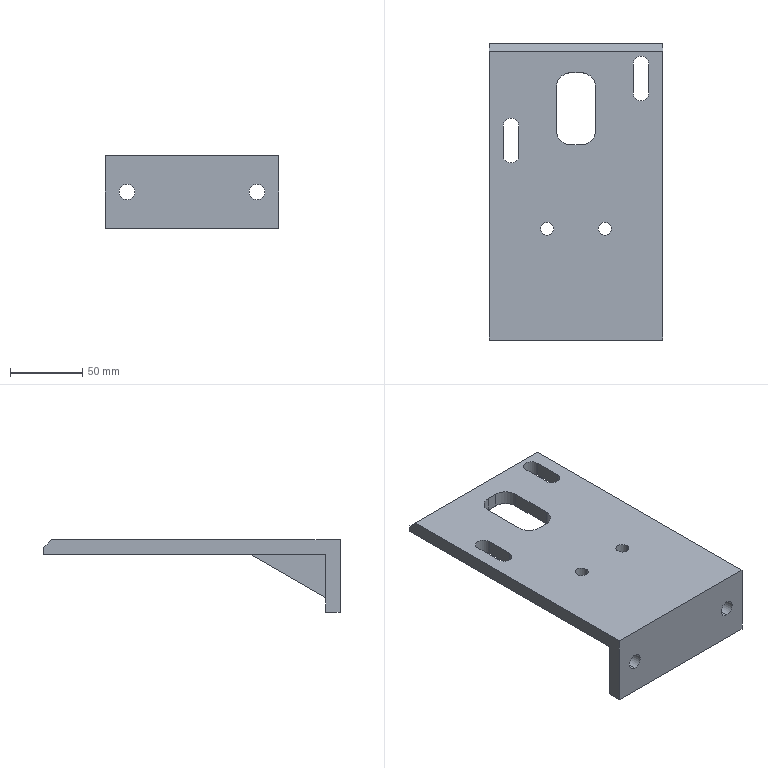NC program | NX | posted with a generic post | part box 120 x 205 x 50 mm
Lines 7209 to 8234 of 11006:
(ZLEVEL_PROFILE_COPY_1 , TOOL : D6)
N14404 T12 M6
N14406 G54
N14408 G17 G0 G90 X-88.106 Y29.874 B0. C0. S5000 M3
N14410 G43 Z30. H12
N14412 Z-10.85
N14414 G41 G94 G1 X-88.2 Y29.84 F1000. D12
N14416 X-89.1 Y29.321
N14418 G3 X-89.4 Y28.801 R0.6
N14420 G1 Y27.639
N14422 G3 X-88.8 Y27.621 R0.6
N14424 G1 X-87.999 Y28.052
N14426 G40
N14428 X-87.92 Y28.114
N14430 G0 X-88.106 Y30.399 Z-11.2
N14432 G41 G1 X-88.2 Y30.365
N14434 X-89.1 Y29.845
N14436 G3 X-89.4 Y29.326 R0.6
N14438 G1 Y27.936
N14440 G3 X-88.81 Y28.043 R0.6
N14442 G1 X-88.114 Y28.631
N14444 G40
N14446 X-88.05 Y28.708
N14448 G0 X-88.106 Y30.78 Z-11.55
N14450 G41 G1 X-88.2 Y30.746
N14452 X-89.1 Y30.226
N14454 G3 X-89.4 Y29.706 R0.6
N14456 G1 Y28.072
N14458 G3 X-88.845 Y28.299 R0.6
N14460 G1 X-88.2 Y29.133
N14462 G40
N14464 X-88.153 Y29.222
N14466 G0 X-88.106 Y31.059 Z-11.9
N14468 G41 G1 X-88.2 Y31.025
N14470 X-89.1 Y30.505
N14472 G3 X-89.4 Y29.986 R0.6
N14474 G1 Y28.099
N14476 X-89.283 Y28.1
N14478 X-89.209
N14480 G3 X-88.689 Y28.4 R0.6
N14482 G1 X-88.2 Y29.248
N14484 G40
N14486 X-88.166 Y29.342
N14488 G0 X-88.106 Y31.245 Z-12.25
N14490 G41 G1 X-88.2 Y31.211
N14492 X-89.1 Y30.692
N14494 G3 X-89.4 Y30.172 R0.6
N14496 G1 Y28.099
N14498 X-89.283 Y28.1
N14500 X-88.603
N14502 G3 X-88.083 Y28.4 R0.6
N14504 G1 X-87.628 Y29.188
N14506 G40
N14508 X-87.594 Y29.282
N14510 G0 X-88.106 Y31.354 Z-12.6
N14512 G41 G1 X-88.2 Y31.32
N14514 X-89.1 Y30.8
N14516 G3 X-89.4 Y30.28 R0.6
N14518 G1 Y28.099
N14520 X-89.283 Y28.1
N14522 X-87.997
N14524 G3 X-87.477 Y28.4 R0.6
N14526 G1 X-87.023 Y29.186
N14528 G40
N14530 X-86.989 Y29.28
N14532 G0 X-88.106 Y31.39 Z-12.95
N14534 G41 G1 X-88.2 Y31.356
N14536 X-89.1 Y30.836
N14538 G3 X-89.4 Y30.316 R0.6
N14540 G1 Y28.099
N14542 X-89.283 Y28.1
N14544 X-87.39
N14546 G3 X-86.871 Y28.4 R0.6
N14548 G1 X-86.417 Y29.186
N14550 G40
N14552 X-86.383 Y29.28
N14554 G0 X-88.106 Y31.39 Z-13.3
N14556 G41 G1 X-88.2 Y31.356
N14558 X-89.1 Y30.836
N14560 G3 X-89.4 Y30.316 R0.6
N14562 G1 Y28.099
N14564 X-89.283 Y28.1
N14566 X-87.184
N14568 G3 X-86.664 Y28.4 R0.6
N14570 G1 X-86.17 Y29.256
N14572 G40
N14574 X-86.136 Y29.35
N14576 G0 X-88.106 Y31.39 Z-13.65
N14578 G41 G1 X-88.2 Y31.356
N14580 X-89.1 Y30.836
N14582 G3 X-89.4 Y30.316 R0.6
N14584 G1 Y28.099
N14586 X-89.283 Y28.1
N14588 X-87.184
N14590 G3 X-86.664 Y28.4 R0.6
N14592 G1 X-86.144 Y29.3
N14594 G40
N14596 X-86.11 Y29.394
N14598 G0 X-88.106 Y31.39 Z-14.
N14600 G41 G1 X-88.2 Y31.356
N14602 X-89.1 Y30.836
N14604 G3 X-89.4 Y30.316 R0.6
N14606 G1 Y28.099
N14608 X-89.283 Y28.1
N14610 X-87.184
N14612 G3 X-86.664 Y28.4 R0.6
N14614 G1 X-86.144 Y29.3
N14616 G40
N14618 X-86.11 Y29.394
N14620 G0 X-88.106 Y31.39 Z-14.35
N14622 G41 G1 X-88.2 Y31.356
N14624 X-89.1 Y30.836
N14626 G3 X-89.4 Y30.316 R0.6
N14628 G1 Y28.099
N14630 X-89.283 Y28.1
N14632 X-87.184
N14634 G3 X-86.664 Y28.4 R0.6
N14636 G1 X-86.144 Y29.3
N14638 G40
N14640 X-86.11 Y29.394
N14642 G0 X-88.106 Y31.39 Z-14.7
N14644 G41 G1 X-88.2 Y31.356
N14646 X-89.1 Y30.836
N14648 G3 X-89.4 Y30.316 R0.6
N14650 G1 Y28.099
N14652 X-89.283 Y28.1
N14654 X-87.184
N14656 G3 X-86.664 Y28.4 R0.6
N14658 G1 X-86.144 Y29.3
N14660 G40
N14662 X-86.11 Y29.394
N14664 G0 X-88.106 Y31.39 Z-15.05
N14666 G41 G1 X-88.2 Y31.356
N14668 X-89.1 Y30.836
N14670 G3 X-89.4 Y30.316 R0.6
N14672 G1 Y28.099
N14674 X-89.283 Y28.1
N14676 X-87.184
N14678 G3 X-86.664 Y28.4 R0.6
N14680 G1 X-86.144 Y29.3
N14682 G40
N14684 X-86.11 Y29.394
N14686 G0 X-88.106 Y31.39 Z-15.4
N14688 G41 G1 X-88.2 Y31.356
N14690 X-89.1 Y30.836
N14692 G3 X-89.4 Y30.316 R0.6
N14694 G1 Y28.099
N14696 X-89.283 Y28.1
N14698 X-87.184
N14700 G3 X-86.664 Y28.4 R0.6
N14702 G1 X-86.144 Y29.3
N14704 G40
N14706 X-86.11 Y29.394
N14708 G0 X-88.106 Y31.39 Z-15.75
N14710 G41 G1 X-88.2 Y31.356
N14712 X-89.1 Y30.836
N14714 G3 X-89.4 Y30.316 R0.6
N14716 G1 Y28.099
N14718 X-89.283 Y28.1
N14720 X-87.184
N14722 G3 X-86.664 Y28.4 R0.6
N14724 G1 X-86.144 Y29.3
N14726 G40
N14728 X-86.11 Y29.394
N14730 G0 X-88.106 Y31.39 Z-16.1
N14732 G41 G1 X-88.2 Y31.356
N14734 X-89.1 Y30.836
N14736 G3 X-89.4 Y30.316 R0.6
N14738 G1 Y28.099
N14740 X-89.283 Y28.1
N14742 X-87.184
N14744 G3 X-86.664 Y28.4 R0.6
N14746 G1 X-86.144 Y29.3
N14748 G40
N14750 X-86.11 Y29.394
N14752 G0 X-88.106 Y31.39 Z-16.45
N14754 G41 G1 X-88.2 Y31.356
N14756 X-89.1 Y30.836
N14758 G3 X-89.4 Y30.316 R0.6
N14760 G1 Y28.099
N14762 X-89.283 Y28.1
N14764 X-87.184
N14766 G3 X-86.664 Y28.4 R0.6
N14768 G1 X-86.144 Y29.3
N14770 G40
N14772 X-86.11 Y29.394
N14774 G0 X-88.106 Y31.39 Z-16.8
N14776 G41 G1 X-88.2 Y31.356
N14778 X-89.1 Y30.836
N14780 G3 X-89.4 Y30.316 R0.6
N14782 G1 Y28.099
N14784 X-89.283 Y28.1
N14786 X-87.184
N14788 G3 X-86.664 Y28.4 R0.6
N14790 G1 X-86.144 Y29.3
N14792 G40
N14794 X-86.11 Y29.394
N14796 G0 X-88.106 Y31.39 Z-17.15
N14798 G41 G1 X-88.2 Y31.356
N14800 X-89.1 Y30.836
N14802 G3 X-89.4 Y30.316 R0.6
N14804 G1 Y28.099
N14806 X-89.283 Y28.1
N14808 X-87.184
N14810 G3 X-86.664 Y28.4 R0.6
N14812 G1 X-86.144 Y29.3
N14814 G40
N14816 X-86.11 Y29.394
N14818 G0 X-88.106 Y31.39 Z-17.5
N14820 G41 G1 X-88.2 Y31.356
N14822 X-89.1 Y30.836
N14824 G3 X-89.4 Y30.316 R0.6
N14826 G1 Y28.099
N14828 X-89.283 Y28.1
N14830 X-87.184
N14832 G3 X-86.664 Y28.4 R0.6
N14834 G1 X-86.144 Y29.3
N14836 G40
N14838 X-86.11 Y29.394
N14840 G0 X-88.106 Y31.39 Z-17.85
N14842 G41 G1 X-88.2 Y31.356
N14844 X-89.1 Y30.836
N14846 G3 X-89.4 Y30.316 R0.6
N14848 G1 Y28.099
N14850 X-89.283 Y28.1
N14852 X-87.184
N14854 G3 X-86.664 Y28.4 R0.6
N14856 G1 X-86.144 Y29.3
N14858 G40
N14860 X-86.11 Y29.394
N14862 G0 X-88.106 Y31.39 Z-18.2
N14864 G41 G1 X-88.2 Y31.356
N14866 X-89.1 Y30.836
N14868 G3 X-89.4 Y30.316 R0.6
N14870 G1 Y28.099
N14872 X-89.283 Y28.1
N14874 X-87.184
N14876 G3 X-86.664 Y28.4 R0.6
N14878 G1 X-86.144 Y29.3
N14880 G40
N14882 X-86.11 Y29.394
N14884 G0 X-88.106 Y31.39 Z-18.55
N14886 G41 G1 X-88.2 Y31.356
N14888 X-89.1 Y30.836
N14890 G3 X-89.4 Y30.316 R0.6
N14892 G1 Y28.099
N14894 X-89.283 Y28.1
N14896 X-87.184
N14898 G3 X-86.664 Y28.4 R0.6
N14900 G1 X-86.144 Y29.3
N14902 G40
N14904 X-86.11 Y29.394
N14906 G0 X-88.106 Y31.39 Z-18.9
N14908 G41 G1 X-88.2 Y31.356
N14910 X-89.1 Y30.836
N14912 G3 X-89.4 Y30.316 R0.6
N14914 G1 Y28.099
N14916 X-89.283 Y28.1
N14918 X-87.184
N14920 G3 X-86.664 Y28.4 R0.6
N14922 G1 X-86.144 Y29.3
N14924 G40
N14926 X-86.11 Y29.394
N14928 G0 X-88.106 Y31.39 Z-19.25
N14930 G41 G1 X-88.2 Y31.356
N14932 X-89.1 Y30.836
N14934 G3 X-89.4 Y30.316 R0.6
N14936 G1 Y28.099
N14938 X-89.283 Y28.1
N14940 X-87.184
N14942 G3 X-86.664 Y28.4 R0.6
N14944 G1 X-86.144 Y29.3
N14946 G40
N14948 X-86.11 Y29.394
N14950 G0 X-88.106 Y31.39 Z-19.6
N14952 G41 G1 X-88.2 Y31.356
N14954 X-89.1 Y30.836
N14956 G3 X-89.4 Y30.316 R0.6
N14958 G1 Y28.099
N14960 X-89.283 Y28.1
N14962 X-87.184
N14964 G3 X-86.664 Y28.4 R0.6
N14966 G1 X-86.144 Y29.3
N14968 G40
N14970 X-86.11 Y29.394
N14972 G0 X-88.106 Y31.39 Z-19.95
N14974 G41 G1 X-88.2 Y31.356
N14976 X-89.1 Y30.836
N14978 G3 X-89.4 Y30.316 R0.6
N14980 G1 Y28.099
N14982 X-89.283 Y28.1
N14984 X-87.184
N14986 G3 X-86.664 Y28.4 R0.6
N14988 G1 X-86.144 Y29.3
N14990 G40
N14992 X-86.11 Y29.394
N14994 G0 X-88.106 Y31.39 Z-20.3
N14996 G41 G1 X-88.2 Y31.356
N14998 X-89.1 Y30.836
N15000 G3 X-89.4 Y30.316 R0.6
N15002 G1 Y28.099
N15004 X-89.283 Y28.1
N15006 X-87.184
N15008 G3 X-86.664 Y28.4 R0.6
N15010 G1 X-86.144 Y29.3
N15012 G40
N15014 X-86.11 Y29.394
N15016 G0 X-88.106 Y31.39 Z-20.65
N15018 G41 G1 X-88.2 Y31.356
N15020 X-89.1 Y30.836
N15022 G3 X-89.4 Y30.316 R0.6
N15024 G1 Y28.099
N15026 X-89.283 Y28.1
N15028 X-87.184
N15030 G3 X-86.664 Y28.4 R0.6
N15032 G1 X-86.144 Y29.3
N15034 G40
N15036 X-86.11 Y29.394
N15038 G0 X-88.106 Y31.39 Z-21.
N15040 G41 G1 X-88.2 Y31.356
N15042 X-89.1 Y30.836
N15044 G3 X-89.4 Y30.316 R0.6
N15046 G1 Y28.099
N15048 X-89.283 Y28.1
N15050 X-87.184
N15052 G3 X-86.664 Y28.4 R0.6
N15054 G1 X-86.144 Y29.3
N15056 G40
N15058 X-86.11 Y29.394
N15060 G0 X-88.106 Y31.39 Z-21.35
N15062 G41 G1 X-88.2 Y31.356
N15064 X-89.1 Y30.836
N15066 G3 X-89.4 Y30.316 R0.6
N15068 G1 Y28.099
N15070 X-89.283 Y28.1
N15072 X-87.184
N15074 G3 X-86.664 Y28.4 R0.6
N15076 G1 X-86.144 Y29.3
N15078 G40
N15080 X-86.11 Y29.394
N15082 G0 X-88.106 Y31.39 Z-21.7
N15084 G41 G1 X-88.2 Y31.356
N15086 X-89.1 Y30.836
N15088 G3 X-89.4 Y30.316 R0.6
N15090 G1 Y28.099
N15092 X-89.283 Y28.1
N15094 X-87.184
N15096 G3 X-86.664 Y28.4 R0.6
N15098 G1 X-86.144 Y29.3
N15100 G40
N15102 X-86.11 Y29.394
N15104 G0 X-88.106 Y31.39 Z-22.05
N15106 G41 G1 X-88.2 Y31.356
N15108 X-89.1 Y30.836
N15110 G3 X-89.4 Y30.316 R0.6
N15112 G1 Y28.099
N15114 X-89.283 Y28.1
N15116 X-87.184
N15118 G3 X-86.664 Y28.4 R0.6
N15120 G1 X-86.144 Y29.3
N15122 G40
N15124 X-86.11 Y29.394
N15126 G0 X-88.106 Y31.39 Z-22.4
N15128 G41 G1 X-88.2 Y31.356
N15130 X-89.1 Y30.836
N15132 G3 X-89.4 Y30.316 R0.6
N15134 G1 Y28.099
N15136 X-89.283 Y28.1
N15138 X-87.184
N15140 G3 X-86.664 Y28.4 R0.6
N15142 G1 X-86.144 Y29.3
N15144 G40
N15146 X-86.11 Y29.394
N15148 G0 X-88.106 Y31.39 Z-22.75
N15150 G41 G1 X-88.2 Y31.356
N15152 X-89.1 Y30.836
N15154 G3 X-89.4 Y30.316 R0.6
N15156 G1 Y28.099
N15158 X-89.283 Y28.1
N15160 X-87.184
N15162 G3 X-86.664 Y28.4 R0.6
N15164 G1 X-86.144 Y29.3
N15166 G40
N15168 X-86.11 Y29.394
N15170 G0 X-88.106 Y31.39 Z-23.1
N15172 G41 G1 X-88.2 Y31.356
N15174 X-89.1 Y30.836
N15176 G3 X-89.4 Y30.316 R0.6
N15178 G1 Y28.099
N15180 X-89.283 Y28.1
N15182 X-87.184
N15184 G3 X-86.664 Y28.4 R0.6
N15186 G1 X-86.144 Y29.3
N15188 G40
N15190 X-86.11 Y29.394
N15192 G0 X-88.106 Y31.39 Z-23.45
N15194 G41 G1 X-88.2 Y31.356
N15196 X-89.1 Y30.836
N15198 G3 X-89.4 Y30.316 R0.6
N15200 G1 Y28.1
N15202 X-89.283
N15204 X-87.184
N15206 G3 X-86.664 Y28.4 R0.6
N15208 G1 X-86.144 Y29.3
N15210 G40
N15212 X-86.11 Y29.394
N15214 G0 X-88.106 Y31.39 Z-23.8
N15216 G41 G1 X-88.2 Y31.356
N15218 X-89.1 Y30.836
N15220 G3 X-89.4 Y30.316 R0.6
N15222 G1 Y28.1
N15224 X-89.283
N15226 X-87.184
N15228 G3 X-86.664 Y28.4 R0.6
N15230 G1 X-86.144 Y29.3
N15232 G40
N15234 X-86.11 Y29.394
N15236 G0 X-88.106 Y31.39 Z-24.15
N15238 G41 G1 X-88.2 Y31.356
N15240 X-89.1 Y30.836
N15242 G3 X-89.4 Y30.316 R0.6
N15244 G1 Y28.1
N15246 X-89.283
N15248 X-87.184
N15250 G3 X-86.664 Y28.4 R0.6
N15252 G1 X-86.144 Y29.3
N15254 G40
N15256 X-86.11 Y29.394
N15258 G0 X-88.106 Y31.39 Z-24.5
N15260 G41 G1 X-88.2 Y31.356
N15262 X-89.1 Y30.836
N15264 G3 X-89.4 Y30.316 R0.6
N15266 G1 Y28.1
N15268 X-89.283
N15270 X-87.184
N15272 G3 X-86.664 Y28.4 R0.6
N15274 G1 X-86.144 Y29.3
N15276 G40
N15278 X-86.11 Y29.394
N15280 G0 X-88.106 Y31.39 Z-24.85
N15282 G41 G1 X-88.2 Y31.356
N15284 X-89.1 Y30.836
N15286 G3 X-89.4 Y30.316 R0.6
N15288 G1 Y28.1
N15290 X-89.283
N15292 X-87.184
N15294 G3 X-86.664 Y28.4 R0.6
N15296 G1 X-86.144 Y29.3
N15298 G40
N15300 X-86.11 Y29.394
N15302 G0 X-88.106 Y31.39 Z-25.2
N15304 G41 G1 X-88.2 Y31.356
N15306 X-89.1 Y30.836
N15308 G3 X-89.4 Y30.316 R0.6
N15310 G1 Y28.1
N15312 X-89.283
N15314 X-87.184
N15316 G3 X-86.664 Y28.4 R0.6
N15318 G1 X-86.144 Y29.3
N15320 G40
N15322 X-86.11 Y29.394
N15324 G0 X-88.106 Y31.39 Z-25.55
N15326 G41 G1 X-88.2 Y31.356
N15328 X-89.1 Y30.836
N15330 G3 X-89.4 Y30.316 R0.6
N15332 G1 Y28.1
N15334 X-89.283
N15336 X-87.184
N15338 G3 X-86.664 Y28.4 R0.6
N15340 G1 X-86.144 Y29.3
N15342 G40
N15344 X-86.11 Y29.394
N15346 G0 X-88.106 Y31.39 Z-25.9
N15348 G41 G1 X-88.2 Y31.356
N15350 X-89.1 Y30.836
N15352 G3 X-89.4 Y30.316 R0.6
N15354 G1 Y28.1
N15356 X-89.283
N15358 X-87.184
N15360 G3 X-86.664 Y28.4 R0.6
N15362 G1 X-86.144 Y29.3
N15364 G40
N15366 X-86.11 Y29.394
N15368 G0 X-88.106 Y31.39 Z-26.25
N15370 G41 G1 X-88.2 Y31.356
N15372 X-89.1 Y30.836
N15374 G3 X-89.4 Y30.316 R0.6
N15376 G1 Y28.1
N15378 X-89.283
N15380 X-87.184
N15382 G3 X-86.664 Y28.4 R0.6
N15384 G1 X-86.144 Y29.3
N15386 G40
N15388 X-86.11 Y29.394
N15390 G0 X-88.106 Y31.39 Z-26.6
N15392 G41 G1 X-88.2 Y31.356
N15394 X-89.1 Y30.836
N15396 G3 X-89.4 Y30.316 R0.6
N15398 G1 Y28.1
N15400 X-89.283
N15402 X-87.184
N15404 G3 X-86.664 Y28.4 R0.6
N15406 G1 X-86.144 Y29.3
N15408 G40
N15410 X-86.11 Y29.394
N15412 G0 X-88.106 Y31.39 Z-26.95
N15414 G41 G1 X-88.2 Y31.356
N15416 X-89.1 Y30.836
N15418 G3 X-89.4 Y30.316 R0.6
N15420 G1 Y28.1
N15422 X-89.283
N15424 X-87.184
N15426 G3 X-86.664 Y28.4 R0.6
N15428 G1 X-86.144 Y29.3
N15430 G40
N15432 X-86.11 Y29.394
N15434 G0 X-88.106 Y31.39 Z-27.3
N15436 G41 G1 X-88.2 Y31.356
N15438 X-89.1 Y30.836
N15440 G3 X-89.4 Y30.316 R0.6
N15442 G1 Y28.1
N15444 X-89.283
N15446 X-87.184
N15448 G3 X-86.664 Y28.4 R0.6
N15450 G1 X-86.144 Y29.3
N15452 G40
N15454 X-86.11 Y29.394
N15456 G0 X-88.106 Y31.39 Z-27.65
N15458 G41 G1 X-88.2 Y31.356
N15460 X-89.1 Y30.836
N15462 G3 X-89.4 Y30.316 R0.6
N15464 G1 Y28.1
N15466 X-89.283
N15468 X-87.184
N15470 G3 X-86.664 Y28.4 R0.6
N15472 G1 X-86.144 Y29.3
N15474 G40
N15476 X-86.11 Y29.394
N15478 G0 X-88.106 Y31.39 Z-28.
N15480 G41 G1 X-88.2 Y31.356
N15482 X-89.1 Y30.836
N15484 G3 X-89.4 Y30.316 R0.6
N15486 G1 Y28.1
N15488 X-89.283
N15490 X-87.184
N15492 G3 X-86.664 Y28.4 R0.6
N15494 G1 X-86.144 Y29.3
N15496 G40
N15498 X-86.11 Y29.394
N15500 G0 X-88.106 Y31.39 Z-28.35
N15502 G41 G1 X-88.2 Y31.356
N15504 X-89.1 Y30.836
N15506 G3 X-89.4 Y30.316 R0.6
N15508 G1 Y28.1
N15510 X-89.283
N15512 X-87.184
N15514 G3 X-86.664 Y28.4 R0.6
N15516 G1 X-86.144 Y29.3
N15518 G40
N15520 X-86.11 Y29.394
N15522 G0 X-88.106 Y31.39 Z-28.7
N15524 G41 G1 X-88.2 Y31.356
N15526 X-89.1 Y30.836
N15528 G3 X-89.4 Y30.316 R0.6
N15530 G1 Y28.1
N15532 X-89.283
N15534 X-87.184
N15536 G3 X-86.664 Y28.4 R0.6
N15538 G1 X-86.144 Y29.3
N15540 G40
N15542 X-86.11 Y29.394
N15544 G0 X-88.106 Y31.39 Z-29.05
N15546 G41 G1 X-88.2 Y31.356
N15548 X-89.1 Y30.836
N15550 G3 X-89.4 Y30.316 R0.6
N15552 G1 Y28.1
N15554 X-89.283
N15556 X-87.184
N15558 G3 X-86.664 Y28.4 R0.6
N15560 G1 X-86.144 Y29.3
N15562 G40
N15564 X-86.11 Y29.394
N15566 G0 X-88.106 Y31.39 Z-29.4
N15568 G41 G1 X-88.2 Y31.356
N15570 X-89.1 Y30.836
N15572 G3 X-89.4 Y30.316 R0.6
N15574 G1 Y28.1
N15576 X-89.283
N15578 X-87.184
N15580 G3 X-86.664 Y28.4 R0.6
N15582 G1 X-86.144 Y29.3
N15584 G40
N15586 X-86.11 Y29.394
N15588 G0 X-88.106 Y31.39 Z-29.75
N15590 G41 G1 X-88.2 Y31.356
N15592 X-89.1 Y30.836
N15594 G3 X-89.4 Y30.316 R0.6
N15596 G1 Y28.1
N15598 X-89.283
N15600 X-87.184
N15602 G3 X-86.664 Y28.4 R0.6
N15604 G1 X-86.144 Y29.3
N15606 G40
N15608 X-86.11 Y29.394
N15610 G0 X-88.106 Y31.39 Z-30.1
N15612 G41 G1 X-88.2 Y31.356
N15614 X-89.1 Y30.836
N15616 G3 X-89.4 Y30.316 R0.6
N15618 G1 Y28.1
N15620 X-89.283
N15622 X-87.184
N15624 G3 X-86.664 Y28.4 R0.6
N15626 G1 X-86.144 Y29.3
N15628 G40
N15630 X-86.11 Y29.394
N15632 G0 X-88.106 Y31.39 Z-30.45
N15634 G41 G1 X-88.2 Y31.356
N15636 X-89.1 Y30.836
N15638 G3 X-89.4 Y30.316 R0.6
N15640 G1 Y28.1
N15642 X-89.283
N15644 X-87.184
N15646 G3 X-86.664 Y28.4 R0.6
N15648 G1 X-86.144 Y29.3
N15650 G40
N15652 X-86.11 Y29.394
N15654 G0 X-88.106 Y31.39 Z-30.8
N15656 G41 G1 X-88.2 Y31.356
N15658 X-89.1 Y30.836
N15660 G3 X-89.4 Y30.316 R0.6
N15662 G1 Y28.1
N15664 X-89.283
N15666 X-87.184
N15668 G3 X-86.664 Y28.4 R0.6
N15670 G1 X-86.144 Y29.3
N15672 G40
N15674 X-86.11 Y29.394
N15676 G0 X-88.106 Y31.39 Z-31.15
N15678 G41 G1 X-88.2 Y31.356
N15680 X-89.1 Y30.836
N15682 G3 X-89.4 Y30.316 R0.6
N15684 G1 Y28.1
N15686 X-89.283
N15688 X-87.184
N15690 G3 X-86.664 Y28.4 R0.6
N15692 G1 X-86.144 Y29.3
N15694 G40
N15696 X-86.11 Y29.394
N15698 G0 X-88.106 Y31.39 Z-31.5
N15700 G41 G1 X-88.2 Y31.356
N15702 X-89.1 Y30.836
N15704 G3 X-89.4 Y30.316 R0.6
N15706 G1 Y28.1
N15708 X-89.283
N15710 X-87.184
N15712 G3 X-86.664 Y28.4 R0.6
N15714 G1 X-86.144 Y29.3
N15716 G40
N15718 X-86.11 Y29.394
N15720 G0 X-88.106 Y31.39 Z-31.85
N15722 G41 G1 X-88.2 Y31.356
N15724 X-89.1 Y30.836
N15726 G3 X-89.4 Y30.316 R0.6
N15728 G1 Y28.1
N15730 X-89.283
N15732 X-87.184
N15734 G3 X-86.664 Y28.4 R0.6
N15736 G1 X-86.144 Y29.3
N15738 G40
N15740 X-86.11 Y29.394
N15742 G0 X-88.106 Y31.39 Z-32.2
N15744 G41 G1 X-88.2 Y31.356
N15746 X-89.1 Y30.836
N15748 G3 X-89.4 Y30.316 R0.6
N15750 G1 Y28.1
N15752 X-89.283
N15754 X-87.184
N15756 G3 X-86.664 Y28.4 R0.6
N15758 G1 X-86.144 Y29.3
N15760 G40
N15762 X-86.11 Y29.394
N15764 G0 X-88.106 Y31.39 Z-32.55
N15766 G41 G1 X-88.2 Y31.356
N15768 X-89.1 Y30.836
N15770 G3 X-89.4 Y30.316 R0.6
N15772 G1 Y28.1
N15774 X-89.283
N15776 X-87.184
N15778 G3 X-86.664 Y28.4 R0.6
N15780 G1 X-86.144 Y29.3
N15782 G40
N15784 X-86.11 Y29.394
N15786 G0 X-88.106 Y31.39 Z-32.9
N15788 G41 G1 X-88.2 Y31.356
N15790 X-89.1 Y30.836
N15792 G3 X-89.4 Y30.316 R0.6
N15794 G1 Y28.1
N15796 X-89.283
N15798 X-87.184
N15800 G3 X-86.664 Y28.4 R0.6
N15802 G1 X-86.144 Y29.3
N15804 G40
N15806 X-86.11 Y29.394
N15808 G0 X-88.106 Y31.39 Z-33.25
N15810 G41 G1 X-88.2 Y31.356
N15812 X-89.1 Y30.836
N15814 G3 X-89.4 Y30.316 R0.6
N15816 G1 Y28.1
N15818 X-87.184
N15820 G3 X-86.664 Y28.4 R0.6
N15822 G1 X-86.144 Y29.3
N15824 G40
N15826 X-86.11 Y29.394
N15828 G0 X-88.106 Y31.39 Z-33.6
N15830 G41 G1 X-88.2 Y31.356
N15832 X-89.1 Y30.836
N15834 G3 X-89.4 Y30.316 R0.6
N15836 G1 Y28.1
N15838 X-87.184
N15840 G3 X-86.664 Y28.4 R0.6
N15842 G1 X-86.144 Y29.3
N15844 G40
N15846 X-86.11 Y29.394
N15848 G0 X-88.106 Y31.39 Z-33.95
N15850 G41 G1 X-88.2 Y31.356
N15852 X-89.1 Y30.836
N15854 G3 X-89.4 Y30.316 R0.6
N15856 G1 Y28.1
N15858 X-87.184
N15860 G3 X-86.664 Y28.4 R0.6
N15862 G1 X-86.144 Y29.3
N15864 G40
N15866 X-86.11 Y29.394
N15868 G0 X-88.106 Y31.39 Z-34.3
N15870 G41 G1 X-88.2 Y31.356
N15872 X-89.1 Y30.836
N15874 G3 X-89.4 Y30.316 R0.6
N15876 G1 Y28.1
N15878 X-87.184
N15880 G3 X-86.664 Y28.4 R0.6
N15882 G1 X-86.144 Y29.3
N15884 G40
N15886 X-86.11 Y29.394
N15888 G0 X-88.106 Y31.39 Z-34.65
N15890 G41 G1 X-88.2 Y31.356
N15892 X-89.1 Y30.836
N15894 G3 X-89.4 Y30.316 R0.6
N15896 G1 Y28.1
N15898 X-87.184
N15900 G3 X-86.664 Y28.4 R0.6
N15902 G1 X-86.144 Y29.3
N15904 G40
N15906 X-86.11 Y29.394
N15908 G0 X-88.106 Y31.39 Z-35.
N15910 G41 G1 X-88.2 Y31.356
N15912 X-89.1 Y30.836
N15914 G3 X-89.4 Y30.316 R0.6
N15916 G1 Y28.1
N15918 X-87.184
N15920 G3 X-86.664 Y28.4 R0.6
N15922 G1 X-86.144 Y29.3
N15924 G40
N15926 X-86.11 Y29.394
N15928 G0 X-88.106 Y31.39 Z-35.35
N15930 G41 G1 X-88.2 Y31.356
N15932 X-89.1 Y30.836
N15934 G3 X-89.4 Y30.316 R0.6
N15936 G1 Y28.1
N15938 X-87.184
N15940 G3 X-86.664 Y28.4 R0.6
N15942 G1 X-86.144 Y29.3
N15944 G40
N15946 X-86.11 Y29.394
N15948 G0 X-88.106 Y31.39 Z-35.7
N15950 G41 G1 X-88.2 Y31.356
N15952 X-89.1 Y30.836
N15954 G3 X-89.4 Y30.316 R0.6
N15956 G1 Y28.1
N15958 X-87.184
N15960 G3 X-86.664 Y28.4 R0.6
N15962 G1 X-86.144 Y29.3
N15964 G40
N15966 X-86.11 Y29.394
N15968 G0 X-88.106 Y31.39 Z-36.05
N15970 G41 G1 X-88.2 Y31.356
N15972 X-89.1 Y30.836
N15974 G3 X-89.4 Y30.316 R0.6
N15976 G1 Y28.1
N15978 X-87.184
N15980 G3 X-86.664 Y28.4 R0.6
N15982 G1 X-86.144 Y29.3
N15984 G40
N15986 X-86.11 Y29.394
N15988 G0 X-88.106 Y31.39 Z-36.4
N15990 G41 G1 X-88.2 Y31.356
N15992 X-89.1 Y30.836
N15994 G3 X-89.4 Y30.316 R0.6
N15996 G1 Y28.1
N15998 X-87.184
N16000 G3 X-86.664 Y28.4 R0.6
N16002 G1 X-86.144 Y29.3
N16004 G40
N16006 X-86.11 Y29.394
N16008 G0 X-88.106 Y31.39 Z-36.75
N16010 G41 G1 X-88.2 Y31.356
N16012 X-89.1 Y30.836
N16014 G3 X-89.4 Y30.316 R0.6
N16016 G1 Y28.1
N16018 X-87.184
N16020 G3 X-86.664 Y28.4 R0.6
N16022 G1 X-86.144 Y29.3
N16024 G40
N16026 X-86.11 Y29.394
N16028 G0 X-88.106 Y31.39 Z-37.1
N16030 G41 G1 X-88.2 Y31.356
N16032 X-89.1 Y30.836
N16034 G3 X-89.4 Y30.316 R0.6
N16036 G1 Y28.1
N16038 X-87.184
N16040 G3 X-86.664 Y28.4 R0.6
N16042 G1 X-86.144 Y29.3
N16044 G40
N16046 X-86.11 Y29.394
N16048 G0 X-88.106 Y31.39 Z-37.45
N16050 G41 G1 X-88.2 Y31.356
N16052 X-89.1 Y30.836
N16054 G3 X-89.4 Y30.316 R0.6
N16056 G1 Y28.1
N16058 X-87.184
N16060 G3 X-86.664 Y28.4 R0.6
N16062 G1 X-86.144 Y29.3
N16064 G40
N16066 X-86.11 Y29.394
N16068 G0 X-88.106 Y31.39 Z-37.8
N16070 G41 G1 X-88.2 Y31.356
N16072 X-89.1 Y30.836
N16074 G3 X-89.4 Y30.316 R0.6
N16076 G1 Y28.1
N16078 X-87.184
N16080 G3 X-86.664 Y28.4 R0.6
N16082 G1 X-86.144 Y29.3
N16084 G40
N16086 X-86.11 Y29.394
N16088 G0 X-88.106 Y31.39 Z-38.15
N16090 G41 G1 X-88.2 Y31.356
N16092 X-89.1 Y30.836
N16094 G3 X-89.4 Y30.316 R0.6
N16096 G1 Y28.1
N16098 X-87.184
N16100 G3 X-86.664 Y28.4 R0.6
N16102 G1 X-86.144 Y29.3
N16104 G40
N16106 X-86.11 Y29.394
N16108 G0 X-88.106 Y31.39 Z-38.5
N16110 G41 G1 X-88.2 Y31.356
N16112 X-89.1 Y30.836
N16114 G3 X-89.4 Y30.316 R0.6
N16116 G1 Y28.1
N16118 X-87.184
N16120 G3 X-86.664 Y28.4 R0.6
N16122 G1 X-86.144 Y29.3
N16124 G40
N16126 X-86.11 Y29.394
N16128 G0 X-88.106 Y31.39 Z-38.85
N16130 G41 G1 X-88.2 Y31.356
N16132 X-89.1 Y30.836
N16134 G3 X-89.4 Y30.316 R0.6
N16136 G1 Y28.1
N16138 X-87.184
N16140 G3 X-86.664 Y28.4 R0.6
N16142 G1 X-86.144 Y29.3
N16144 G40
N16146 X-86.11 Y29.394
N16148 G0 X-88.106 Y31.39 Z-39.138
N16150 G41 G1 X-88.2 Y31.356
N16152 X-89.1 Y30.836
N16154 G3 X-89.4 Y30.316 R0.6
N16156 G1 Y28.1
N16158 X-87.184
N16160 G3 X-86.664 Y28.4 R0.6
N16162 G1 X-86.144 Y29.3
N16164 G40
N16166 X-86.11 Y29.394
N16168 G0 X-88.106 Y31.39 Z-39.425
N16170 G41 G1 X-88.2 Y31.356
N16172 X-89.1 Y30.836
N16174 G3 X-89.4 Y30.316 R0.6
N16176 G1 Y28.1
N16178 X-87.184
N16180 G3 X-86.664 Y28.4 R0.6
N16182 G1 X-86.144 Y29.3
N16184 G40
N16186 X-86.11 Y29.394
N16188 G0 X-88.106 Y31.39 Z-39.713
N16190 G41 G1 X-88.2 Y31.356
N16192 X-89.1 Y30.836
N16194 G3 X-89.4 Y30.316 R0.6
N16196 G1 Y28.1
N16198 X-87.184
N16200 G3 X-86.664 Y28.4 R0.6
N16202 G1 X-86.144 Y29.3
N16204 G40
N16206 X-86.11 Y29.394
N16208 G0 X-88.106 Y31.39 Z-40.
N16210 G41 G1 X-88.2 Y31.356
N16212 X-89.1 Y30.836
N16214 G3 X-89.4 Y30.316 R0.6
N16216 G1 Y28.1
N16218 X-87.184
N16220 G3 X-86.664 Y28.4 R0.6
N16222 G1 X-86.144 Y29.3
N16224 G40
N16226 X-86.11 Y29.394
N16228 G0 Z30.
N16230 X-87.917 Y11.886
N16232 Z-10.85
N16234 G41 G1 X-87.996 Y11.947
N16236 X-88.8 Y12.374
N16238 G3 X-89.4 Y12.353 R0.6
N16240 G1 Y11.197
N16242 G3 X-89.1 Y10.678 R0.6
N16244 G1 X-88.2 Y10.158
N16246 G40
N16248 X-88.106 Y10.124
N16250 G0 X-88.055 Y11.289 Z-11.2
N16252 G41 G1 X-88.119 Y11.367
N16254 X-88.81 Y11.959
N16256 G3 X-89.4 Y12.069 R0.6
N16258 G1 Y10.677
N16260 G3 X-89.1 Y10.157 R0.6
N16262 G1 X-88.2 Y9.637
N16264 G40
N16266 X-88.106 Y9.603
N16268 G0 X-88.154 Y10.778 Z-11.55
N16270 G41 G1 X-88.2 Y10.866
N16272 X-88.845 Y11.7
N16274 G3 X-89.4 Y11.928 R0.6
N16276 G1 Y10.293
N16278 G3 X-89.1 Y9.773 R0.6
N16280 G1 X-88.2 Y9.253
N16282 G40
N16284 X-88.106 Y9.219
N16286 G0 X-88.166 Y10.658 Z-11.9
N16288 G41 G1 X-88.2 Y10.752
N16290 X-88.689 Y11.6
N16292 G3 X-89.209 Y11.9 R0.6
N16294 G1 X-89.283
N16296 X-89.4 Y11.901
N16298 Y10.015
N16300 G3 X-89.1 Y9.496 R0.6
N16302 G1 X-88.2 Y8.976
N16304 G40
N16306 X-88.106 Y8.942
N16308 G0 X-87.594 Y10.718 Z-12.25
N16310 G41 G1 X-87.628 Y10.812
N16312 X-88.083 Y11.6
N16314 G3 X-88.603 Y11.9 R0.6
N16316 G1 X-89.283
N16318 X-89.4 Y11.901
N16320 Y9.829
N16322 G3 X-89.1 Y9.309 R0.6
N16324 G1 X-88.2 Y8.789
N16326 G40
N16328 X-88.106 Y8.755
N16330 G0 X-86.988 Y10.718 Z-12.6
N16332 G41 G1 X-87.022 Y10.812
N16334 X-87.477 Y11.6
N16336 G3 X-87.997 Y11.9 R0.6
N16338 G1 X-89.283
N16340 X-89.4 Y11.901
N16342 Y9.719
N16344 G3 X-89.1 Y9.2 R0.6
N16346 G1 X-88.2 Y8.68
N16348 G40
N16350 X-88.106 Y8.646
N16352 G0 X-86.382 Y10.718 Z-12.95
N16354 G41 G1 X-86.416 Y10.812
N16356 X-86.871 Y11.6
N16358 G3 X-87.39 Y11.9 R0.6
N16360 G1 X-89.283
N16362 X-89.4 Y11.901
N16364 Y9.684
N16366 G3 X-89.1 Y9.164 R0.6
N16368 G1 X-88.2 Y8.644
N16370 G40
N16372 X-88.106 Y8.61
N16374 G0 X-86.136 Y10.65 Z-13.3
N16376 G41 G1 X-86.17 Y10.744
N16378 X-86.664 Y11.6
N16380 G3 X-87.184 Y11.9 R0.6
N16382 G1 X-89.283
N16384 X-89.4 Y11.901
N16386 Y9.684
N16388 G3 X-89.1 Y9.164 R0.6
N16390 G1 X-88.2 Y8.644
N16392 G40
N16394 X-88.106 Y8.61
N16396 G0 X-86.11 Y10.606 Z-13.65
N16398 G41 G1 X-86.144 Y10.7
N16400 X-86.664 Y11.6
N16402 G3 X-87.184 Y11.9 R0.6
N16404 G1 X-89.283
N16406 X-89.4 Y11.901
N16408 Y9.684
N16410 G3 X-89.1 Y9.164 R0.6
N16412 G1 X-88.2 Y8.644
N16414 G40
N16416 X-88.106 Y8.61
N16418 G0 X-86.11 Y10.606 Z-14.
N16420 G41 G1 X-86.144 Y10.7
N16422 X-86.664 Y11.6
N16424 G3 X-87.184 Y11.9 R0.6
N16426 G1 X-89.283
N16428 X-89.4 Y11.901
N16430 Y9.684
N16432 G3 X-89.1 Y9.164 R0.6
N16434 G1 X-88.2 Y8.644
N16436 G40
N16438 X-88.106 Y8.61
N16440 G0 X-86.11 Y10.606 Z-14.35
N16442 G41 G1 X-86.144 Y10.7
N16444 X-86.664 Y11.6
N16446 G3 X-87.184 Y11.9 R0.6
N16448 G1 X-89.283